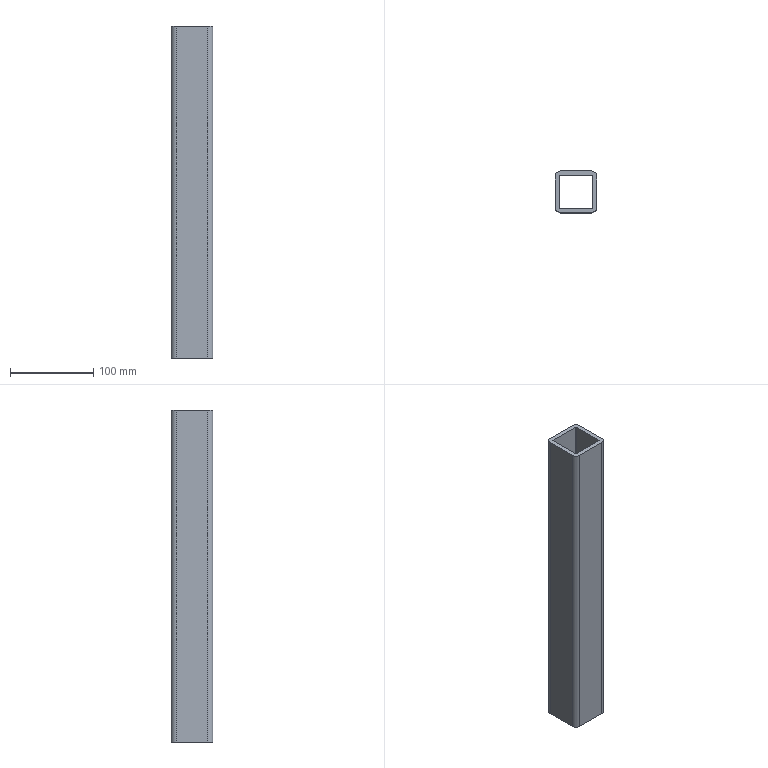Part | SolidWorks | features Extrusion 1 | 1 solid | 18 faces | box 50 x 50 x 400 mm | volume 347982 mm3 | plane 10 | cylinder 8 | commonest cylinder face diameters 2 x4 12 x4
STEP:
#1=CARTESIAN_POINT('',(0.,6.,400.));
#2=VERTEX_POINT('',#1);
#3=CARTESIAN_POINT('',(6.,0.,400.));
#4=VERTEX_POINT('',#3);
#5=CARTESIAN_POINT('',(6.,6.,400.));
#6=DIRECTION('',(0.,0.,1.));
#7=DIRECTION('',(-1.,0.,0.));
#8=AXIS2_PLACEMENT_3D('',#5,#6,#7);
#9=CIRCLE('',#8,6.);
#10=EDGE_CURVE('',#2,#4,#9,.T.);
#11=ORIENTED_EDGE('',*,*,#10,.T.);
#12=CARTESIAN_POINT('',(44.,0.,400.));
#13=VERTEX_POINT('',#12);
#14=CARTESIAN_POINT('',(6.,0.,400.));
#15=DIRECTION('',(1.,0.,0.));
#16=VECTOR('',#15,1000.);
#17=LINE('',#14,#16);
#18=EDGE_CURVE('',#4,#13,#17,.T.);
#19=ORIENTED_EDGE('',*,*,#18,.T.);
#20=CARTESIAN_POINT('',(50.,6.,400.));
#21=VERTEX_POINT('',#20);
#22=CARTESIAN_POINT('',(44.,6.,400.));
#23=DIRECTION('',(0.,0.,1.));
#24=DIRECTION('',(1.,0.,0.));
#25=AXIS2_PLACEMENT_3D('',#22,#23,#24);
#26=CIRCLE('',#25,6.);
#27=EDGE_CURVE('',#13,#21,#26,.T.);
#28=ORIENTED_EDGE('',*,*,#27,.T.);
#29=CARTESIAN_POINT('',(50.,44.,400.));
#30=VERTEX_POINT('',#29);
#31=CARTESIAN_POINT('',(50.,6.,400.));
#32=DIRECTION('',(0.,1.,0.));
#33=VECTOR('',#32,1000.);
#34=LINE('',#31,#33);
#35=EDGE_CURVE('',#21,#30,#34,.T.);
#36=ORIENTED_EDGE('',*,*,#35,.T.);
#37=CARTESIAN_POINT('',(44.,50.,400.));
#38=VERTEX_POINT('',#37);
#39=CARTESIAN_POINT('',(44.,44.,400.));
#40=DIRECTION('',(0.,0.,1.));
#41=DIRECTION('',(-1.,0.,0.));
#42=AXIS2_PLACEMENT_3D('',#39,#40,#41);
#43=CIRCLE('',#42,6.);
#44=EDGE_CURVE('',#30,#38,#43,.T.);
#45=ORIENTED_EDGE('',*,*,#44,.T.);
#46=CARTESIAN_POINT('',(6.,50.,400.));
#47=VERTEX_POINT('',#46);
#48=CARTESIAN_POINT('',(6.,50.,400.));
#49=DIRECTION('',(-1.,0.,0.));
#50=VECTOR('',#49,1000.);
#51=LINE('',#48,#50);
#52=EDGE_CURVE('',#38,#47,#51,.T.);
#53=ORIENTED_EDGE('',*,*,#52,.T.);
#54=CARTESIAN_POINT('',(0.,44.,400.));
#55=VERTEX_POINT('',#54);
#56=CARTESIAN_POINT('',(6.,44.,400.));
#57=DIRECTION('',(0.,0.,1.));
#58=DIRECTION('',(-1.,0.,0.));
#59=AXIS2_PLACEMENT_3D('',#56,#57,#58);
#60=CIRCLE('',#59,6.);
#61=EDGE_CURVE('',#47,#55,#60,.T.);
#62=ORIENTED_EDGE('',*,*,#61,.T.);
#63=CARTESIAN_POINT('',(0.,6.,400.));
#64=DIRECTION('',(0.,-1.,0.));
#65=VECTOR('',#64,1000.);
#66=LINE('',#63,#65);
#67=EDGE_CURVE('',#55,#2,#66,.T.);
#68=ORIENTED_EDGE('',*,*,#67,.T.);
#69=EDGE_LOOP('',(#11,#19,#28,#36,#45,#53,#62,#68));
#70=FACE_OUTER_BOUND('',#69,.T.);
#71=CARTESIAN_POINT('',(6.,45.,400.));
#72=VERTEX_POINT('',#71);
#73=CARTESIAN_POINT('',(5.,44.,400.));
#74=VERTEX_POINT('',#73);
#75=CARTESIAN_POINT('',(6.,44.,400.));
#76=DIRECTION('',(0.,0.,1.));
#77=DIRECTION('',(-1.,0.,0.));
#78=AXIS2_PLACEMENT_3D('',#75,#76,#77);
#79=CIRCLE('',#78,1.);
#80=EDGE_CURVE('',#72,#74,#79,.T.);
#81=ORIENTED_EDGE('',*,*,#80,.F.);
#82=CARTESIAN_POINT('',(44.,45.,400.));
#83=VERTEX_POINT('',#82);
#84=CARTESIAN_POINT('',(6.,45.,400.));
#85=DIRECTION('',(-1.,0.,0.));
#86=VECTOR('',#85,1000.);
#87=LINE('',#84,#86);
#88=EDGE_CURVE('',#83,#72,#87,.T.);
#89=ORIENTED_EDGE('',*,*,#88,.F.);
#90=CARTESIAN_POINT('',(45.,44.,400.));
#91=VERTEX_POINT('',#90);
#92=CARTESIAN_POINT('',(44.,44.,400.));
#93=DIRECTION('',(0.,0.,1.));
#94=DIRECTION('',(-1.,0.,0.));
#95=AXIS2_PLACEMENT_3D('',#92,#93,#94);
#96=CIRCLE('',#95,1.);
#97=EDGE_CURVE('',#91,#83,#96,.T.);
#98=ORIENTED_EDGE('',*,*,#97,.F.);
#99=CARTESIAN_POINT('',(45.,6.,400.));
#100=VERTEX_POINT('',#99);
#101=CARTESIAN_POINT('',(45.,6.,400.));
#102=DIRECTION('',(0.,1.,0.));
#103=VECTOR('',#102,1000.);
#104=LINE('',#101,#103);
#105=EDGE_CURVE('',#100,#91,#104,.T.);
#106=ORIENTED_EDGE('',*,*,#105,.F.);
#107=CARTESIAN_POINT('',(44.,5.,400.));
#108=VERTEX_POINT('',#107);
#109=CARTESIAN_POINT('',(44.,6.,400.));
#110=DIRECTION('',(0.,0.,1.));
#111=DIRECTION('',(1.,0.,0.));
#112=AXIS2_PLACEMENT_3D('',#109,#110,#111);
#113=CIRCLE('',#112,1.);
#114=EDGE_CURVE('',#108,#100,#113,.T.);
#115=ORIENTED_EDGE('',*,*,#114,.F.);
#116=CARTESIAN_POINT('',(6.,5.,400.));
#117=VERTEX_POINT('',#116);
#118=CARTESIAN_POINT('',(6.,5.,400.));
#119=DIRECTION('',(1.,0.,0.));
#120=VECTOR('',#119,1000.);
#121=LINE('',#118,#120);
#122=EDGE_CURVE('',#117,#108,#121,.T.);
#123=ORIENTED_EDGE('',*,*,#122,.F.);
#124=CARTESIAN_POINT('',(5.,6.,400.));
#125=VERTEX_POINT('',#124);
#126=CARTESIAN_POINT('',(6.,6.,400.));
#127=DIRECTION('',(0.,0.,1.));
#128=DIRECTION('',(-1.,0.,0.));
#129=AXIS2_PLACEMENT_3D('',#126,#127,#128);
#130=CIRCLE('',#129,1.);
#131=EDGE_CURVE('',#125,#117,#130,.T.);
#132=ORIENTED_EDGE('',*,*,#131,.F.);
#133=CARTESIAN_POINT('',(5.,6.,400.));
#134=DIRECTION('',(0.,-1.,0.));
#135=VECTOR('',#134,1000.);
#136=LINE('',#133,#135);
#137=EDGE_CURVE('',#74,#125,#136,.T.);
#138=ORIENTED_EDGE('',*,*,#137,.F.);
#139=EDGE_LOOP('',(#81,#89,#98,#106,#115,#123,#132,#138));
#140=FACE_BOUND('',#139,.T.);
#141=CARTESIAN_POINT('',(6.,6.,400.));
#142=DIRECTION('',(0.,0.,-1.));
#143=DIRECTION('',(-1.,0.,0.));
#144=AXIS2_PLACEMENT_3D('',#141,#142,#143);
#145=PLANE('',#144);
#146=ADVANCED_FACE('',(#70,#140),#145,.F.);
#147=CARTESIAN_POINT('',(0.,6.,0.));
#148=VERTEX_POINT('',#147);
#149=CARTESIAN_POINT('',(6.,0.,0.));
#150=VERTEX_POINT('',#149);
#151=CARTESIAN_POINT('',(6.,6.,0.));
#152=DIRECTION('',(0.,0.,1.));
#153=DIRECTION('',(-1.,0.,0.));
#154=AXIS2_PLACEMENT_3D('',#151,#152,#153);
#155=CIRCLE('',#154,6.);
#156=EDGE_CURVE('',#148,#150,#155,.T.);
#157=ORIENTED_EDGE('',*,*,#156,.F.);
#158=CARTESIAN_POINT('',(0.,44.,0.));
#159=VERTEX_POINT('',#158);
#160=CARTESIAN_POINT('',(0.,6.,0.));
#161=DIRECTION('',(0.,-1.,0.));
#162=VECTOR('',#161,1000.);
#163=LINE('',#160,#162);
#164=EDGE_CURVE('',#159,#148,#163,.T.);
#165=ORIENTED_EDGE('',*,*,#164,.F.);
#166=CARTESIAN_POINT('',(6.,50.,0.));
#167=VERTEX_POINT('',#166);
#168=CARTESIAN_POINT('',(6.,44.,0.));
#169=DIRECTION('',(0.,0.,1.));
#170=DIRECTION('',(-1.,0.,0.));
#171=AXIS2_PLACEMENT_3D('',#168,#169,#170);
#172=CIRCLE('',#171,6.);
#173=EDGE_CURVE('',#167,#159,#172,.T.);
#174=ORIENTED_EDGE('',*,*,#173,.F.);
#175=CARTESIAN_POINT('',(44.,50.,0.));
#176=VERTEX_POINT('',#175);
#177=CARTESIAN_POINT('',(6.,50.,0.));
#178=DIRECTION('',(-1.,0.,0.));
#179=VECTOR('',#178,1000.);
#180=LINE('',#177,#179);
#181=EDGE_CURVE('',#176,#167,#180,.T.);
#182=ORIENTED_EDGE('',*,*,#181,.F.);
#183=CARTESIAN_POINT('',(50.,44.,0.));
#184=VERTEX_POINT('',#183);
#185=CARTESIAN_POINT('',(44.,44.,0.));
#186=DIRECTION('',(0.,0.,1.));
#187=DIRECTION('',(-1.,0.,0.));
#188=AXIS2_PLACEMENT_3D('',#185,#186,#187);
#189=CIRCLE('',#188,6.);
#190=EDGE_CURVE('',#184,#176,#189,.T.);
#191=ORIENTED_EDGE('',*,*,#190,.F.);
#192=CARTESIAN_POINT('',(50.,6.,0.));
#193=VERTEX_POINT('',#192);
#194=CARTESIAN_POINT('',(50.,6.,0.));
#195=DIRECTION('',(0.,1.,0.));
#196=VECTOR('',#195,1000.);
#197=LINE('',#194,#196);
#198=EDGE_CURVE('',#193,#184,#197,.T.);
#199=ORIENTED_EDGE('',*,*,#198,.F.);
#200=CARTESIAN_POINT('',(44.,0.,0.));
#201=VERTEX_POINT('',#200);
#202=CARTESIAN_POINT('',(44.,6.,0.));
#203=DIRECTION('',(0.,0.,1.));
#204=DIRECTION('',(1.,0.,0.));
#205=AXIS2_PLACEMENT_3D('',#202,#203,#204);
#206=CIRCLE('',#205,6.);
#207=EDGE_CURVE('',#201,#193,#206,.T.);
#208=ORIENTED_EDGE('',*,*,#207,.F.);
#209=CARTESIAN_POINT('',(6.,0.,0.));
#210=DIRECTION('',(1.,0.,0.));
#211=VECTOR('',#210,1000.);
#212=LINE('',#209,#211);
#213=EDGE_CURVE('',#150,#201,#212,.T.);
#214=ORIENTED_EDGE('',*,*,#213,.F.);
#215=EDGE_LOOP('',(#157,#165,#174,#182,#191,#199,#208,#214));
#216=FACE_OUTER_BOUND('',#215,.T.);
#217=CARTESIAN_POINT('',(44.,45.,0.));
#218=VERTEX_POINT('',#217);
#219=CARTESIAN_POINT('',(6.,45.,0.));
#220=VERTEX_POINT('',#219);
#221=CARTESIAN_POINT('',(6.,45.,0.));
#222=DIRECTION('',(-1.,0.,0.));
#223=VECTOR('',#222,1000.);
#224=LINE('',#221,#223);
#225=EDGE_CURVE('',#218,#220,#224,.T.);
#226=ORIENTED_EDGE('',*,*,#225,.T.);
#227=CARTESIAN_POINT('',(5.,44.,0.));
#228=VERTEX_POINT('',#227);
#229=CARTESIAN_POINT('',(6.,44.,0.));
#230=DIRECTION('',(0.,0.,1.));
#231=DIRECTION('',(-1.,0.,0.));
#232=AXIS2_PLACEMENT_3D('',#229,#230,#231);
#233=CIRCLE('',#232,1.);
#234=EDGE_CURVE('',#220,#228,#233,.T.);
#235=ORIENTED_EDGE('',*,*,#234,.T.);
#236=CARTESIAN_POINT('',(5.,6.,0.));
#237=VERTEX_POINT('',#236);
#238=CARTESIAN_POINT('',(5.,6.,0.));
#239=DIRECTION('',(0.,-1.,0.));
#240=VECTOR('',#239,1000.);
#241=LINE('',#238,#240);
#242=EDGE_CURVE('',#228,#237,#241,.T.);
#243=ORIENTED_EDGE('',*,*,#242,.T.);
#244=CARTESIAN_POINT('',(6.,5.,0.));
#245=VERTEX_POINT('',#244);
#246=CARTESIAN_POINT('',(6.,6.,0.));
#247=DIRECTION('',(0.,0.,1.));
#248=DIRECTION('',(-1.,0.,0.));
#249=AXIS2_PLACEMENT_3D('',#246,#247,#248);
#250=CIRCLE('',#249,1.);
#251=EDGE_CURVE('',#237,#245,#250,.T.);
#252=ORIENTED_EDGE('',*,*,#251,.T.);
#253=CARTESIAN_POINT('',(44.,5.,0.));
#254=VERTEX_POINT('',#253);
#255=CARTESIAN_POINT('',(6.,5.,0.));
#256=DIRECTION('',(1.,0.,0.));
#257=VECTOR('',#256,1000.);
#258=LINE('',#255,#257);
#259=EDGE_CURVE('',#245,#254,#258,.T.);
#260=ORIENTED_EDGE('',*,*,#259,.T.);
#261=CARTESIAN_POINT('',(45.,6.,0.));
#262=VERTEX_POINT('',#261);
#263=CARTESIAN_POINT('',(44.,6.,0.));
#264=DIRECTION('',(0.,0.,1.));
#265=DIRECTION('',(1.,0.,0.));
#266=AXIS2_PLACEMENT_3D('',#263,#264,#265);
#267=CIRCLE('',#266,1.);
#268=EDGE_CURVE('',#254,#262,#267,.T.);
#269=ORIENTED_EDGE('',*,*,#268,.T.);
#270=CARTESIAN_POINT('',(45.,44.,0.));
#271=VERTEX_POINT('',#270);
#272=CARTESIAN_POINT('',(45.,6.,0.));
#273=DIRECTION('',(0.,1.,0.));
#274=VECTOR('',#273,1000.);
#275=LINE('',#272,#274);
#276=EDGE_CURVE('',#262,#271,#275,.T.);
#277=ORIENTED_EDGE('',*,*,#276,.T.);
#278=CARTESIAN_POINT('',(44.,44.,0.));
#279=DIRECTION('',(0.,0.,1.));
#280=DIRECTION('',(-1.,0.,0.));
#281=AXIS2_PLACEMENT_3D('',#278,#279,#280);
#282=CIRCLE('',#281,1.);
#283=EDGE_CURVE('',#271,#218,#282,.T.);
#284=ORIENTED_EDGE('',*,*,#283,.T.);
#285=EDGE_LOOP('',(#226,#235,#243,#252,#260,#269,#277,#284));
#286=FACE_BOUND('',#285,.T.);
#287=CARTESIAN_POINT('',(6.,6.,0.));
#288=DIRECTION('',(0.,0.,-1.));
#289=DIRECTION('',(-1.,0.,0.));
#290=AXIS2_PLACEMENT_3D('',#287,#288,#289);
#291=PLANE('',#290);
#292=ADVANCED_FACE('',(#216,#286),#291,.T.);
#293=ORIENTED_EDGE('',*,*,#156,.T.);
#294=CARTESIAN_POINT('',(6.,0.,400.));
#295=DIRECTION('',(0.,0.,-1.));
#296=VECTOR('',#295,1000.);
#297=LINE('',#294,#296);
#298=EDGE_CURVE('',#4,#150,#297,.T.);
#299=ORIENTED_EDGE('',*,*,#298,.F.);
#300=ORIENTED_EDGE('',*,*,#10,.F.);
#301=CARTESIAN_POINT('',(0.,6.,400.));
#302=DIRECTION('',(0.,0.,-1.));
#303=VECTOR('',#302,1000.);
#304=LINE('',#301,#303);
#305=EDGE_CURVE('',#2,#148,#304,.T.);
#306=ORIENTED_EDGE('',*,*,#305,.T.);
#307=EDGE_LOOP('',(#293,#299,#300,#306));
#308=FACE_OUTER_BOUND('',#307,.T.);
#309=CARTESIAN_POINT('',(6.,6.,400.));
#310=DIRECTION('',(0.,0.,-1.));
#311=DIRECTION('',(-1.,0.,0.));
#312=AXIS2_PLACEMENT_3D('',#309,#310,#311);
#313=CYLINDRICAL_SURFACE('',#312,6.);
#314=ADVANCED_FACE('',(#308),#313,.T.);
#315=ORIENTED_EDGE('',*,*,#213,.T.);
#316=CARTESIAN_POINT('',(44.,0.,400.));
#317=DIRECTION('',(0.,0.,-1.));
#318=VECTOR('',#317,1000.);
#319=LINE('',#316,#318);
#320=EDGE_CURVE('',#13,#201,#319,.T.);
#321=ORIENTED_EDGE('',*,*,#320,.F.);
#322=ORIENTED_EDGE('',*,*,#18,.F.);
#323=ORIENTED_EDGE('',*,*,#298,.T.);
#324=EDGE_LOOP('',(#315,#321,#322,#323));
#325=FACE_OUTER_BOUND('',#324,.T.);
#326=CARTESIAN_POINT('',(6.,0.,400.));
#327=DIRECTION('',(0.,1.,0.));
#328=DIRECTION('',(0.,0.,1.));
#329=AXIS2_PLACEMENT_3D('',#326,#327,#328);
#330=PLANE('',#329);
#331=ADVANCED_FACE('',(#325),#330,.F.);
#332=ORIENTED_EDGE('',*,*,#207,.T.);
#333=CARTESIAN_POINT('',(50.,6.,400.));
#334=DIRECTION('',(0.,0.,-1.));
#335=VECTOR('',#334,1000.);
#336=LINE('',#333,#335);
#337=EDGE_CURVE('',#21,#193,#336,.T.);
#338=ORIENTED_EDGE('',*,*,#337,.F.);
#339=ORIENTED_EDGE('',*,*,#27,.F.);
#340=ORIENTED_EDGE('',*,*,#320,.T.);
#341=EDGE_LOOP('',(#332,#338,#339,#340));
#342=FACE_OUTER_BOUND('',#341,.T.);
#343=CARTESIAN_POINT('',(44.,6.,400.));
#344=DIRECTION('',(0.,0.,-1.));
#345=DIRECTION('',(-1.,0.,0.));
#346=AXIS2_PLACEMENT_3D('',#343,#344,#345);
#347=CYLINDRICAL_SURFACE('',#346,6.);
#348=ADVANCED_FACE('',(#342),#347,.T.);
#349=ORIENTED_EDGE('',*,*,#198,.T.);
#350=CARTESIAN_POINT('',(50.,44.,400.));
#351=DIRECTION('',(0.,0.,-1.));
#352=VECTOR('',#351,1000.);
#353=LINE('',#350,#352);
#354=EDGE_CURVE('',#30,#184,#353,.T.);
#355=ORIENTED_EDGE('',*,*,#354,.F.);
#356=ORIENTED_EDGE('',*,*,#35,.F.);
#357=ORIENTED_EDGE('',*,*,#337,.T.);
#358=EDGE_LOOP('',(#349,#355,#356,#357));
#359=FACE_OUTER_BOUND('',#358,.T.);
#360=CARTESIAN_POINT('',(50.,6.,400.));
#361=DIRECTION('',(-1.,0.,0.));
#362=DIRECTION('',(0.,0.,1.));
#363=AXIS2_PLACEMENT_3D('',#360,#361,#362);
#364=PLANE('',#363);
#365=ADVANCED_FACE('',(#359),#364,.F.);
#366=ORIENTED_EDGE('',*,*,#190,.T.);
#367=CARTESIAN_POINT('',(44.,50.,400.));
#368=DIRECTION('',(0.,0.,-1.));
#369=VECTOR('',#368,1000.);
#370=LINE('',#367,#369);
#371=EDGE_CURVE('',#38,#176,#370,.T.);
#372=ORIENTED_EDGE('',*,*,#371,.F.);
#373=ORIENTED_EDGE('',*,*,#44,.F.);
#374=ORIENTED_EDGE('',*,*,#354,.T.);
#375=EDGE_LOOP('',(#366,#372,#373,#374));
#376=FACE_OUTER_BOUND('',#375,.T.);
#377=CARTESIAN_POINT('',(44.,44.,400.));
#378=DIRECTION('',(0.,0.,-1.));
#379=DIRECTION('',(-1.,0.,0.));
#380=AXIS2_PLACEMENT_3D('',#377,#378,#379);
#381=CYLINDRICAL_SURFACE('',#380,6.);
#382=ADVANCED_FACE('',(#376),#381,.T.);
#383=ORIENTED_EDGE('',*,*,#181,.T.);
#384=CARTESIAN_POINT('',(6.,50.,400.));
#385=DIRECTION('',(0.,0.,-1.));
#386=VECTOR('',#385,1000.);
#387=LINE('',#384,#386);
#388=EDGE_CURVE('',#47,#167,#387,.T.);
#389=ORIENTED_EDGE('',*,*,#388,.F.);
#390=ORIENTED_EDGE('',*,*,#52,.F.);
#391=ORIENTED_EDGE('',*,*,#371,.T.);
#392=EDGE_LOOP('',(#383,#389,#390,#391));
#393=FACE_OUTER_BOUND('',#392,.T.);
#394=CARTESIAN_POINT('',(6.,50.,400.));
#395=DIRECTION('',(0.,-1.,0.));
#396=DIRECTION('',(0.,0.,-1.));
#397=AXIS2_PLACEMENT_3D('',#394,#395,#396);
#398=PLANE('',#397);
#399=ADVANCED_FACE('',(#393),#398,.F.);
#400=ORIENTED_EDGE('',*,*,#173,.T.);
#401=CARTESIAN_POINT('',(0.,44.,400.));
#402=DIRECTION('',(0.,0.,-1.));
#403=VECTOR('',#402,1000.);
#404=LINE('',#401,#403);
#405=EDGE_CURVE('',#55,#159,#404,.T.);
#406=ORIENTED_EDGE('',*,*,#405,.F.);
#407=ORIENTED_EDGE('',*,*,#61,.F.);
#408=ORIENTED_EDGE('',*,*,#388,.T.);
#409=EDGE_LOOP('',(#400,#406,#407,#408));
#410=FACE_OUTER_BOUND('',#409,.T.);
#411=CARTESIAN_POINT('',(6.,44.,400.));
#412=DIRECTION('',(0.,0.,-1.));
#413=DIRECTION('',(-1.,0.,0.));
#414=AXIS2_PLACEMENT_3D('',#411,#412,#413);
#415=CYLINDRICAL_SURFACE('',#414,6.);
#416=ADVANCED_FACE('',(#410),#415,.T.);
#417=ORIENTED_EDGE('',*,*,#164,.T.);
#418=ORIENTED_EDGE('',*,*,#305,.F.);
#419=ORIENTED_EDGE('',*,*,#67,.F.);
#420=ORIENTED_EDGE('',*,*,#405,.T.);
#421=EDGE_LOOP('',(#417,#418,#419,#420));
#422=FACE_OUTER_BOUND('',#421,.T.);
#423=CARTESIAN_POINT('',(0.,6.,400.));
#424=DIRECTION('',(1.,0.,0.));
#425=DIRECTION('',(0.,0.,-1.));
#426=AXIS2_PLACEMENT_3D('',#423,#424,#425);
#427=PLANE('',#426);
#428=ADVANCED_FACE('',(#422),#427,.F.);
#429=ORIENTED_EDGE('',*,*,#234,.F.);
#430=CARTESIAN_POINT('',(6.,45.,400.));
#431=DIRECTION('',(0.,0.,-1.));
#432=VECTOR('',#431,1000.);
#433=LINE('',#430,#432);
#434=EDGE_CURVE('',#72,#220,#433,.T.);
#435=ORIENTED_EDGE('',*,*,#434,.F.);
#436=ORIENTED_EDGE('',*,*,#80,.T.);
#437=CARTESIAN_POINT('',(5.,44.,400.));
#438=DIRECTION('',(0.,0.,-1.));
#439=VECTOR('',#438,1000.);
#440=LINE('',#437,#439);
#441=EDGE_CURVE('',#74,#228,#440,.T.);
#442=ORIENTED_EDGE('',*,*,#441,.T.);
#443=EDGE_LOOP('',(#429,#435,#436,#442));
#444=FACE_OUTER_BOUND('',#443,.T.);
#445=CARTESIAN_POINT('',(6.,44.,400.));
#446=DIRECTION('',(0.,0.,-1.));
#447=DIRECTION('',(-1.,0.,0.));
#448=AXIS2_PLACEMENT_3D('',#445,#446,#447);
#449=CYLINDRICAL_SURFACE('',#448,1.);
#450=ADVANCED_FACE('',(#444),#449,.F.);
#451=ORIENTED_EDGE('',*,*,#242,.F.);
#452=ORIENTED_EDGE('',*,*,#441,.F.);
#453=ORIENTED_EDGE('',*,*,#137,.T.);
#454=CARTESIAN_POINT('',(5.,6.,400.));
#455=DIRECTION('',(0.,0.,-1.));
#456=VECTOR('',#455,1000.);
#457=LINE('',#454,#456);
#458=EDGE_CURVE('',#125,#237,#457,.T.);
#459=ORIENTED_EDGE('',*,*,#458,.T.);
#460=EDGE_LOOP('',(#451,#452,#453,#459));
#461=FACE_OUTER_BOUND('',#460,.T.);
#462=CARTESIAN_POINT('',(5.,6.,400.));
#463=DIRECTION('',(1.,0.,0.));
#464=DIRECTION('',(0.,1.,0.));
#465=AXIS2_PLACEMENT_3D('',#462,#463,#464);
#466=PLANE('',#465);
#467=ADVANCED_FACE('',(#461),#466,.T.);
#468=ORIENTED_EDGE('',*,*,#251,.F.);
#469=ORIENTED_EDGE('',*,*,#458,.F.);
#470=ORIENTED_EDGE('',*,*,#131,.T.);
#471=CARTESIAN_POINT('',(6.,5.,400.));
#472=DIRECTION('',(0.,0.,-1.));
#473=VECTOR('',#472,1000.);
#474=LINE('',#471,#473);
#475=EDGE_CURVE('',#117,#245,#474,.T.);
#476=ORIENTED_EDGE('',*,*,#475,.T.);
#477=EDGE_LOOP('',(#468,#469,#470,#476));
#478=FACE_OUTER_BOUND('',#477,.T.);
#479=CARTESIAN_POINT('',(6.,6.,400.));
#480=DIRECTION('',(0.,0.,-1.));
#481=DIRECTION('',(-1.,0.,0.));
#482=AXIS2_PLACEMENT_3D('',#479,#480,#481);
#483=CYLINDRICAL_SURFACE('',#482,1.);
#484=ADVANCED_FACE('',(#478),#483,.F.);
#485=ORIENTED_EDGE('',*,*,#259,.F.);
#486=ORIENTED_EDGE('',*,*,#475,.F.);
#487=ORIENTED_EDGE('',*,*,#122,.T.);
#488=CARTESIAN_POINT('',(44.,5.,400.));
#489=DIRECTION('',(0.,0.,-1.));
#490=VECTOR('',#489,1000.);
#491=LINE('',#488,#490);
#492=EDGE_CURVE('',#108,#254,#491,.T.);
#493=ORIENTED_EDGE('',*,*,#492,.T.);
#494=EDGE_LOOP('',(#485,#486,#487,#493));
#495=FACE_OUTER_BOUND('',#494,.T.);
#496=CARTESIAN_POINT('',(6.,5.,400.));
#497=DIRECTION('',(0.,1.,0.));
#498=DIRECTION('',(-1.,0.,0.));
#499=AXIS2_PLACEMENT_3D('',#496,#497,#498);
#500=PLANE('',#499);
#501=ADVANCED_FACE('',(#495),#500,.T.);
#502=ORIENTED_EDGE('',*,*,#268,.F.);
#503=ORIENTED_EDGE('',*,*,#492,.F.);
#504=ORIENTED_EDGE('',*,*,#114,.T.);
#505=CARTESIAN_POINT('',(45.,6.,400.));
#506=DIRECTION('',(0.,0.,-1.));
#507=VECTOR('',#506,1000.);
#508=LINE('',#505,#507);
#509=EDGE_CURVE('',#100,#262,#508,.T.);
#510=ORIENTED_EDGE('',*,*,#509,.T.);
#511=EDGE_LOOP('',(#502,#503,#504,#510));
#512=FACE_OUTER_BOUND('',#511,.T.);
#513=CARTESIAN_POINT('',(44.,6.,400.));
#514=DIRECTION('',(0.,0.,-1.));
#515=DIRECTION('',(-1.,0.,0.));
#516=AXIS2_PLACEMENT_3D('',#513,#514,#515);
#517=CYLINDRICAL_SURFACE('',#516,1.);
#518=ADVANCED_FACE('',(#512),#517,.F.);
#519=ORIENTED_EDGE('',*,*,#276,.F.);
#520=ORIENTED_EDGE('',*,*,#509,.F.);
#521=ORIENTED_EDGE('',*,*,#105,.T.);
#522=CARTESIAN_POINT('',(45.,44.,400.));
#523=DIRECTION('',(0.,0.,-1.));
#524=VECTOR('',#523,1000.);
#525=LINE('',#522,#524);
#526=EDGE_CURVE('',#91,#271,#525,.T.);
#527=ORIENTED_EDGE('',*,*,#526,.T.);
#528=EDGE_LOOP('',(#519,#520,#521,#527));
#529=FACE_OUTER_BOUND('',#528,.T.);
#530=CARTESIAN_POINT('',(45.,6.,400.));
#531=DIRECTION('',(-1.,0.,0.));
#532=DIRECTION('',(0.,0.,1.));
#533=AXIS2_PLACEMENT_3D('',#530,#531,#532);
#534=PLANE('',#533);
#535=ADVANCED_FACE('',(#529),#534,.T.);
#536=ORIENTED_EDGE('',*,*,#283,.F.);
#537=ORIENTED_EDGE('',*,*,#526,.F.);
#538=ORIENTED_EDGE('',*,*,#97,.T.);
#539=CARTESIAN_POINT('',(44.,45.,400.));
#540=DIRECTION('',(0.,0.,-1.));
#541=VECTOR('',#540,1000.);
#542=LINE('',#539,#541);
#543=EDGE_CURVE('',#83,#218,#542,.T.);
#544=ORIENTED_EDGE('',*,*,#543,.T.);
#545=EDGE_LOOP('',(#536,#537,#538,#544));
#546=FACE_OUTER_BOUND('',#545,.T.);
#547=CARTESIAN_POINT('',(44.,44.,400.));
#548=DIRECTION('',(0.,0.,-1.));
#549=DIRECTION('',(-1.,0.,0.));
#550=AXIS2_PLACEMENT_3D('',#547,#548,#549);
#551=CYLINDRICAL_SURFACE('',#550,1.);
#552=ADVANCED_FACE('',(#546),#551,.F.);
#553=ORIENTED_EDGE('',*,*,#225,.F.);
#554=ORIENTED_EDGE('',*,*,#543,.F.);
#555=ORIENTED_EDGE('',*,*,#88,.T.);
#556=ORIENTED_EDGE('',*,*,#434,.T.);
#557=EDGE_LOOP('',(#553,#554,#555,#556));
#558=FACE_OUTER_BOUND('',#557,.T.);
#559=CARTESIAN_POINT('',(6.,45.,400.));
#560=DIRECTION('',(0.,-1.,0.));
#561=DIRECTION('',(0.,0.,-1.));
#562=AXIS2_PLACEMENT_3D('',#559,#560,#561);
#563=PLANE('',#562);
#564=ADVANCED_FACE('',(#558),#563,.T.);
#565=CLOSED_SHELL('',(#146,#292,#314,#331,#348,#365,#382,#399,#416,#428,#450,#467,#484,#501,#518,#535,#552,#564));
#566=MANIFOLD_SOLID_BREP('',#565);
#567=CARTESIAN_POINT('',(0.,0.,0.));
#568=DIRECTION('',(0.,0.,1.));
#569=DIRECTION('',(1.,0.,0.));
#570=AXIS2_PLACEMENT_3D('',#567,#568,#569);
#571=(LENGTH_UNIT()NAMED_UNIT(*)SI_UNIT(.MILLI.,.METRE.));
#572=UNCERTAINTY_MEASURE_WITH_UNIT(LENGTH_MEASURE(0.00001),#571,'','');
#573=(NAMED_UNIT(*)PLANE_ANGLE_UNIT()SI_UNIT($,.RADIAN.));
#574=(NAMED_UNIT(*)SI_UNIT($,.STERADIAN.)SOLID_ANGLE_UNIT());
#575=(GEOMETRIC_REPRESENTATION_CONTEXT(3)GLOBAL_UNCERTAINTY_ASSIGNED_CONTEXT((#572))GLOBAL_UNIT_ASSIGNED_CONTEXT((#571,#573,#574))REPRESENTATION_CONTEXT('',''));
#576=ADVANCED_BREP_SHAPE_REPRESENTATION('',(#566,#570),#575);